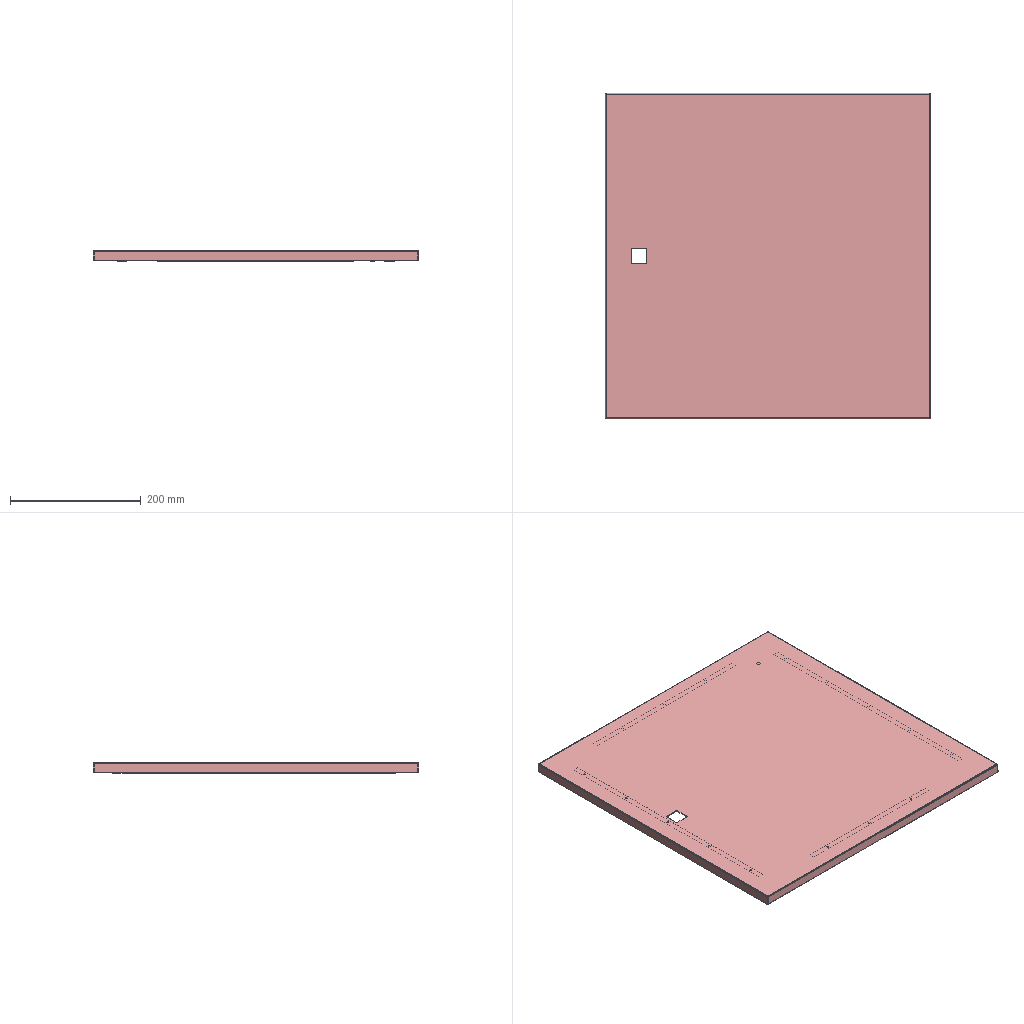Assembly | SolidWorks | 6 different items | 7 placed | box 499 x 498 x 17 mm
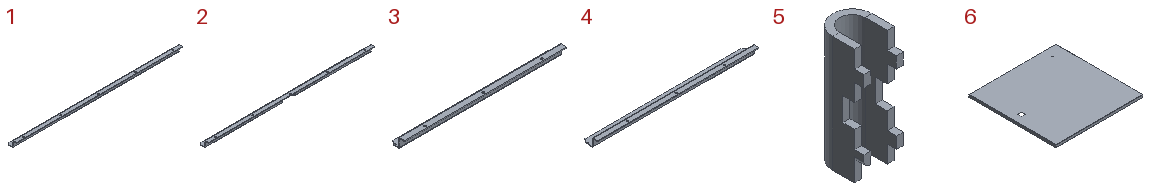Parts list (item | quantity | size | volume | features):
1 | x1 | 400 x 23.5 x 15 mm | 21483 mm3 | features LPattern 4, EdgeFlange 2, ICE 2, Chamfer 1, FlatPattern 1, SMBaseFlange 1, SheetMetal 1
2 | x1 | 400 x 23.5 x 15 mm | 20417 mm3 | features LPattern 4, ICE 3, EdgeFlange 2, Chamfer 1, FlatPattern 1, SMBaseFlange 1, SheetMetal 1
3 | x1 | 250 x 23.5 x 15 mm | 13407 mm3 | features LPattern 4, EdgeFlange 2, ICE 2, Chamfer 1, FlatPattern 1, SMBaseFlange 1, SheetMetal 1
4 | x1 | 300 x 28.5 x 15 mm | 18353 mm3 | features LPattern 4, EdgeFlange 2, ICE 2, Chamfer 1, FlatPattern 1, SMBaseFlange 1, SheetMetal 1
5 | x2 | 8.5 x 11 x 25 mm | 759.819 mm3 | features Fillet 1, FlatPattern 1, ICE 1, SMBaseFlange 1, SheetMetal 1
6 | x1 | 498 x 498 x 16.5 mm | 410662 mm3 | features ICE 3, LPattern 3, EdgeFlange 2, FlatPattern 1, SMBaseFlange 1, SheetMetal 1
Mates (type | each side: item.copy, entity, surface, feature):
Coincident | 6.1 face plane Edge-Flange1 | 5.1 face plane Cut-Extrude1
DistanceDim | 5.1 face plane Base-Flange1 | 6.1 face plane Edge-Flange1
DistanceDim | 5.1 face plane Base-Flange1 | 6.1 face plane Edge-Flange2
Coincident | 6.1 face plane Base-Flange1 | 2.1 face plane Edge-Flange2
Coincident | 6.1 face plane Base-Flange1 | 1.1 face plane Edge-Flange2
DistanceDim | 6.1 face plane Edge-Flange1 | 2.1 face plane Edge-Flange1
DistanceDim | 2.1 face plane Cut-Extrude3 | 6.1 face plane Cut-Extrude1
Coincident | 2.1 face plane Edge-Flange2 | 1.1 face plane Edge-Flange1
DistanceDim | 1.1 face plane Edge-Flange1 | 6.1 face plane Edge-Flange1
Coincident | 6.1 face plane Base-Flange1 | 3.1 face plane Edge-Flange2
Width | 6.1 face plane Edge-Flange1 | 6.1 face plane Edge-Flange1 | 3.1 face plane Edge-Flange1 | 3.1 face plane Edge-Flange1
Coincident | 2.1 face plane Base-Flange1 | 3.1 face plane Base-Flange1
Coincident | 6.1 face plane Base-Flange1 | 4.1 face plane Edge-Flange2
Coincident | 2.1 face plane Base-Flange1 | 4.1 face plane Base-Flange1
Width | 6.1 face plane Edge-Flange1 | 6.1 face plane Edge-Flange1 | 4.1 face plane Edge-Flange1 | 4.1 face plane Edge-Flange1